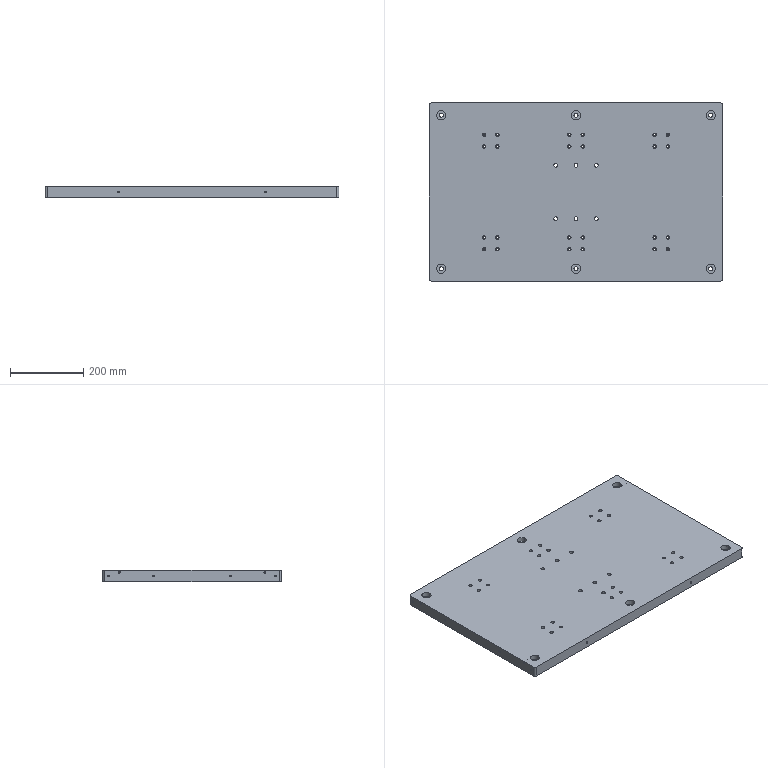NC program | Mastercam | posted with a generic post | part box 800 x 485 x 30 mm
Lines 4969 to 5776 of 13355:
N160 T9 M6
N170 G0 G90 G17 G54 X-108.24 Y-180.7 A0. S7000 M3
N180 G43 H9 Z50. M8
N190 Z1.
N200 G1 Z-.97 F600.
N210 Y-179.75 F3000.
N220 Y-173.741
N230 X-247.218
N240 Y-179.75
N250 G2 X-248.249 Y-180.781 I-1.031 J0.
N260 G1 X-252.509
N270 G2 X-253.541 Y-179.75 I0. J1.031
N280 G1 Y-167.418
N290 X-101.918
N300 Y-179.75
N310 G3 X-100.887 Y-180.781 I1.031 J0.
N320 G1 X-96.627
N330 G3 X-95.595 Y-179.75 I0. J1.031
N340 G1 Y-161.096
N350 X-259.863
N360 Y-179.75
N370 G2 X-260.894 Y-180.781 I-1.031 J0.
N380 G1 X-265.343
N390 G2 X-266.375 Y-179.75 I0. J1.031
N400 G1 X-266.374 Y-154.584
N410 X-89.084
N420 X-89.001 Y-179.75
N430 G3 X-87.972 Y-180.778 I1.031 J.003
N440 G1 X-83.604 Y-180.784
N450 X-83.602
N460 G3 X-82.571 Y-179.753 I0. J1.031
N470 G1 Y-179.75
N480 X-82.646 Y-152.389
N490 X-82.445 Y-148.147
N500 X-273.014
N510 X-272.812 Y-152.389
N520 X-272.888 Y-179.75
N530 G2 X-273.918 Y-180.778 I-1.031 J.003
N540 G1 X-278.098 Y-180.784
N550 X-278.099
N560 G2 X-279.131 Y-179.752 I0. J1.032
N570 G1 Y-179.75
N580 X-279.066 Y-152.389
N590 G3 X-280.436 Y-141.893 I-55.601 J-1.92
N600 G1 X-75.023
N610 G3 X-76.393 Y-152.389 I54.232 J-12.416
N620 G1 Y-179.75
N630 G3 X-75.361 Y-180.781 I1.032 J0.
N640 G1 X-71.477 Y-180.78
N650 G3 X-70.446 Y-179.75 I0. J1.032
N660 G1 X-70.396 Y-150.079
N670 G2 X-66.439 Y-135.985 I38.55 J-3.221
N680 G1 X-289.033
N690 G2 X-284.974 Y-152.389 I-33.033 J-16.878
N700 G1 X-285.029 Y-179.75
N710 G2 X-286.06 Y-180.779 I-1.031 J.002
N720 G1 X-289.089 Y-180.781
N730 G2 X-290.121 Y-179.75 I0. J1.031
N740 G1 X-290.12 Y-152.389
N750 G3 X-291.547 Y-143.256 I-54.5 J-3.836
N760 X-299.139 Y-130.838 I-30.518 J-10.127
N770 G1 X-56.319
N780 G3 X-65.338 Y-152.389 I21.751 J-21.766
N790 G1 X-65.262 Y-179.75
N800 Y-180.7
N810 G0 Z50.
N820 X98.24
N830 Z1.
N840 G1 Z-.97 F600.
N850 Y-179.75 F3000.
N860 Y-173.741
N870 X246.858
N880 Y-179.75
N890 G3 X247.889 Y-180.781 I1.031 J0.
N900 G1 X252.149
N910 G3 X253.18 Y-179.75 I0. J1.031
N920 G1 Y-167.418
N930 X91.918
N940 Y-179.75
N950 G2 X90.887 Y-180.781 I-1.031 J0.
N960 G1 X86.627
N970 G2 X85.595 Y-179.75 I0. J1.031
N980 G1 Y-161.096
N990 X259.503
N1000 Y-179.75
N1010 G3 X260.533 Y-180.781 I1.031 J0.
N1020 G1 X265.065 Y-180.785
N1030 X265.066
N1040 G3 X266.098 Y-179.753 I0. J1.032
N1050 G1 Y-179.75
N1060 X266.014 Y-154.584
N1070 X79.084
N1080 Y-179.75
N1090 G2 X78.053 Y-180.781 I-1.031 J0.
N1100 G1 X73.541 Y-180.782
N1110 G2 X72.51 Y-179.75 I0. J1.032
N1120 G1 X72.523 Y-149.152
N1130 X72.445 Y-148.147
N1140 X272.653
N1150 X272.452 Y-152.389
N1160 X272.527 Y-179.75
N1170 G3 X273.558 Y-180.778 I1.032 J.003
N1180 G1 X277.674 Y-180.781
N1190 G3 X278.705 Y-179.75 I0. J1.031
N1200 G1 Y-152.389
N1210 G2 X280.075 Y-141.893 I55.602 J-1.92
N1220 G1 X65.023
N1230 G2 X66.393 Y-152.389 I-54.232 J-12.416
N1240 G1 Y-179.75
N1250 G2 X65.362 Y-180.781 I-1.032 J0.
N1260 G1 X61.461 Y-180.783
N1270 G2 X60.43 Y-179.752 I0. J1.031
N1280 G1 Y-179.75
N1290 X60.484 Y-152.389
N1300 G3 X56.437 Y-135.985 I-37.292 J-.499
N1310 G1 X288.658
N1320 G3 X284.702 Y-150.079 I34.621 J-17.319
N1330 G1 X284.652 Y-179.75
N1340 Y-179.752
N1350 G3 X285.683 Y-180.783 I1.031 J0.
N1360 G1 X285.685
N1370 X288.785 Y-180.779
N1380 G3 X289.815 Y-179.75 I-.001 J1.031
N1390 G1 X289.887 Y-149.766
N1400 G2 X298.78 Y-130.838 I30.644 J-2.843
N1410 G1 X46.319
N1420 G2 X55.338 Y-152.389 I-21.719 J-21.752
N1430 G1 X55.262 Y-179.75
N1440 G2 X54.232 Y-180.778 I-1.031 J.003
N1450 G1 X51.99 Y-180.781
N1460 X51.989
N1470 G2 X50.958 Y-179.75 I0. J1.031
N1480 G1 Y-152.389
N1490 G3 X49.414 Y-143.661 I-37.021 J-2.047
N1500 X24.964 Y-126.458 I-24.45 J-8.773
N1510 G1 X24.706 Y-126.459
N1520 X-4.941 Y-126.458
N1530 X-35.55 Y-126.469
N1540 G3 X-45.618 Y-128.753 I1.584 J-30.309
N1550 X-60.958 Y-152.389 I10.663 J-23.716
N1560 G1 Y-179.75
N1570 G3 X-59.926 Y-180.781 I1.032 J0.
N1580 G1 X-56.231
N1590 G3 X-55.199 Y-179.75 I0. J1.031
N1600 G1 X-55.2 Y-152.389
N1610 G2 X-42.636 Y-133.739 I20.258 J-.089
N1620 X-35.479 Y-132.227 I8.822 J-24.062
N1630 G1 X-4.941 Y-132.217
N1640 X24.706
N1650 G2 X24.961 Y-132.215 I.255 J-20.226
N1660 X44.628 Y-147.712 I0. J-20.228
N1670 X45.2 Y-152.389 I-23.861 J-5.287
N1680 G1 X45.199 Y-179.75
N1690 G2 X44.168 Y-180.781 I-1.031 J0.
N1700 G1 X38.731
N1710 G2 X37.7 Y-179.75 I0. J1.031
N1720 G1 Y-152.389
N1730 X37.466 Y-150.05
N1740 G3 X24.945 Y-139.714 I-12.521 J-2.416
N1750 X24.706 Y-139.717 I0. J-12.752
N1760 G1 X-4.941
N1770 X-35.387 Y-139.726
N1780 G3 X-38.398 Y-140.192 I.7 J-14.491
N1790 X-47.7 Y-152.389 I3.468 J-12.29
N1800 G1 Y-179.75
N1810 G3 X-46.668 Y-180.781 I1.032 J0.
N1820 G1 X-41.231
N1830 G3 X-40.2 Y-179.75 I0. J1.031
N1840 G1 Y-152.389
N1850 G2 X-38.824 Y-148.893 I5.379 J-.098
N1860 X-36. Y-147.317 I3.89 J-3.654
N1870 G1 X-35.294 Y-147.225
N1880 X-34.589 Y-147.216
N1890 X-4.941
N1900 X24.706
N1910 G2 X24.915 Y-147.212 I.209 J-5.42
N1920 X28.236 Y-148.347 I0. J-5.424
N1930 X30.146 Y-151.683 I-3.335 J-4.125
N1940 G1 X30.2 Y-152.389
N1950 Y-179.8
N1960 G3 X30.208 Y-179.929 I1.031 J0.
N1970 X30.232 Y-180.056 I1.023 J.129
N1980 X30.272 Y-180.179 I.999 J.256
N1990 X30.327 Y-180.296 I.959 J.379
N2000 X30.396 Y-180.405 I.904 J.496
N2010 X30.478 Y-180.505 I.835 J.605
N2020 X30.572 Y-180.594 I.753 J.705
N2030 X30.677 Y-180.67 I.659 J.794
N2040 X30.79 Y-180.732 I.554 J.87
N2050 X30.91 Y-180.78 I.441 J.932
N2060 X31.035 Y-180.812 I.321 J.98
N2070 X31.163 Y-180.829 I.196 J1.012
N2080 X31.231 Y-180.831 I.068 J1.029
N2090 X31.293 Y-180.829 I0. J1.031
N2100 X31.421 Y-180.814 I-.062 J1.029
N2110 X31.546 Y-180.782 I-.19 J1.014
N2120 X31.667 Y-180.735 I-.315 J.982
N2130 G1 X31.741 Y-180.7
N2140 G0 Z50.
N2150 X110.882 Y180.7
N2160 Z1.
N2170 G1 Z-.97 F600.
N2180 Y179.75 F3000.
N2190 G2 X110.885 Y176.337 I-1974.811 J-3.873
N2200 G1 X130. Y173.396
N2210 X171.3 Y179.75
N2220 G3 X171.469 Y179.791 I-.156 J1.019
N2230 X171.628 Y179.859 I-.325 J.978
N2240 X171.773 Y179.953 I-.484 J.91
N2250 X171.901 Y180.07 I-.629 J.816
N2260 X172.008 Y180.206 I-.757 J.699
N2270 X172.09 Y180.359 I-.864 J.563
N2280 X172.145 Y180.523 I-.946 J.41
N2290 X172.172 Y180.694 I-1.001 J.246
N2300 G0 Z50.
N2310 X217.781
N2320 Z1.
N2330 G1 Z-.97 F600.
N2340 G3 X217.808 Y180.523 I1.028 J.075 F3000.
N2350 X217.863 Y180.359 I1.001 J.246
N2360 X217.945 Y180.206 I.946 J.41
N2370 X218.052 Y180.069 I.864 J.563
N2380 X218.179 Y179.953 I.757 J.7
N2390 X218.325 Y179.859 I.63 J.816
N2400 X218.484 Y179.791 I.484 J.91
N2410 X218.653 Y179.75 I.325 J.978
N2420 G1 X234.213 Y177.363
N2430 Y179.75
N2440 G2 X235.244 Y180.781 I1.031 J0.
N2450 G1 X239.504
N2460 G2 X240.535 Y179.75 I0. J-1.031
N2470 G1 Y169.994
N2480 X205.957 Y175.301
N2490 X197.254 Y176.019
N2500 G3 X182.812 Y175.124 I2.943 J-164.466
N2510 G1 X130. Y166.999
N2520 X104.563 Y170.913
N2530 Y179.75
N2540 G3 X103.532 Y180.781 I-1.031 J0.
N2550 G1 X99.272
N2560 G3 X98.24 Y179.75 I0. J-1.031
N2570 G1 Y165.488
N2580 X130. Y160.602
N2590 X183.774 Y168.875
N2600 G2 X197.048 Y169.7 I18.149 J-184.875
N2610 G1 X205.635 Y168.961
N2620 X246.858 Y162.624
N2630 Y179.75
N2640 G2 X247.889 Y180.781 I1.031 J0.
N2650 G1 X252.149
N2660 G2 X253.18 Y179.75 I0. J-1.031
N2670 G1 Y155.255
N2680 X204.749 Y162.701
N2690 X196.841 Y163.381
N2700 G3 X184.735 Y162.626 I8.881 J-239.961
N2710 G1 X130. Y154.205
N2720 X91.918 Y160.064
N2730 Y179.75
N2740 G3 X90.887 Y180.781 I-1.031 J0.
N2750 G1 X86.535 Y180.785
N2760 X86.534
N2770 G3 X85.503 Y179.754 I0. J-1.031
N2780 G1 Y179.75
N2790 X85.595 Y154.64
N2800 X130. Y147.808
N2810 X185.696 Y156.377
N2820 G2 X195.946 Y157.051 I10.25 J-77.614
N2830 X197.341 Y157.038 I0. J-78.288
N2840 G1 X203.862 Y156.441
N2850 X259.688 Y147.857
N2860 X259.58 Y179.75
N2870 Y180.7
N2880 G0 Z50.
N2890 X400.705 Y122.986
N2900 Z1.
N2910 G1 Z-.97 F600.
N2920 G3 X400.464 Y123.049 I-.383 J-.958 F3000.
N2930 X400.322 Y123.059 I-.142 J-1.021
N2940 X400.215 Y123.054 I0. J-1.031
N2950 X399.972 Y122.998 I.107 J-1.026
N2960 X399.75 Y122.886 I.35 J-.97
N2970 G2 X397.083 Y121.27 I-19.748 J29.59
N2980 X399.75 Y120.565 I-10.375 J-44.643
N2990 X400.47 Y119.766 I-.294 J-.989
N3000 G1 X401.109 Y116.344
N3010 G2 X401.127 Y116.154 I-1.013 J-.19
N3020 X400.096 Y115.123 I-1.031 J0.
N3030 X399.75 Y115.183 I0. J1.031
N3040 G3 X398.045 Y115.739 I-11.247 J-31.588
N3050 G1 X394.179 Y116.552
N3060 X358.259 Y122.078
N3070 G3 X364.193 Y122.05 I5.934 J638.917
N3080 X384.148 Y122.362 I0. J638.945
N3090 X395.65 Y126.383 I-5.237 J33.449
N3100 X399.75 Y129.33 I-15.663 J26.112
N3110 G2 X399.851 Y129.406 I.669 J-.785
N3120 X399.962 Y129.47 I.568 J-.861
N3130 X400.079 Y129.519 I.457 J-.925
N3140 X400.202 Y129.553 I.34 J-.974
N3150 X400.327 Y129.572 I.217 J-1.008
N3160 X400.419 Y129.576 I.092 J-1.027
N3170 G1 X400.455 Y129.575
N3180 G2 X400.581 Y129.564 I-.036 J-1.031
N3190 X400.705 Y129.536 I-.162 J-1.019
N3200 G0 Z50.
N3210 X400.7 Y-129.214
N3220 Z1.
N3230 G1 Z-.97 F600.
N3240 X400.181 Y-129.164 F3000.
N3250 G3 X400.082 Y-129.159 I-.099 J-1.026
N3260 X399.963 Y-129.166 I0. J-1.031
N3270 X399.75 Y-129.214 I.119 J-1.024
N3280 G2 X399.667 Y-129.242 I-9.786 J28.75
N3290 X399.75 Y-129.312 I-19.836 J-23.307
N3300 G3 X400.421 Y-129.56 I.671 J.783
N3310 X401.452 Y-128.529 I0. J1.031
N3320 X401.446 Y-128.419 I-1.031 J0.
N3330 G1 X401.12 Y-125.386
N3340 G3 X400.095 Y-124.465 I-1.025 J-.11
N3350 X399.75 Y-124.524 I0. J-1.031
N3360 G2 X390.731 Y-126.442 I-11.76 J33.139
N3370 G1 X350.121 Y-126.458
N3380 X-389.651
N3390 X-390.731 Y-126.442
N3400 G2 X-399.75 Y-124.545 I.751 J25.961
N3410 G3 X-399.882 Y-124.502 I-.388 J-.956
N3420 X-400.02 Y-124.476 I-.256 J-.999
N3430 X-400.138 Y-124.469 I-.118 J-1.025
N3440 X-400.159 Y-124.47 I0. J-1.032
N3450 X-400.298 Y-124.482 I.021 J-1.031
N3460 G1 X-400.7 Y-124.545
N3470 G0 Z50.
N3480 X-400.703 Y-135.412
N3490 Z1.
N3500 G1 Z-.97 F600.
N3510 G3 X-400.572 Y-135.427 I.186 J1.015 F3000.
N3520 X-400.517 Y-135.428 I.055 J1.03
N3530 X-400.441 Y-135.426 I0. J1.031
N3540 X-400.311 Y-135.408 I-.076 J1.029
N3550 X-400.184 Y-135.373 I-.206 J1.011
N3560 X-400.063 Y-135.323 I-.333 J.976
N3570 X-399.948 Y-135.258 I-.454 J.926
N3580 X-399.844 Y-135.179 I-.569 J.861
N3590 X-399.75 Y-135.087 I-.673 J.782
N3600 G2 X-392.359 Y-129.372 I19.351 J-17.391
N3610 X-382.009 Y-126.515 I12.84 J-26.338
N3620 G1 X-350.474 Y-126.458
N3630 X-320.474
N3640 G2 X-295.778 Y-144.408 I-.033 J-26.009
N3650 X-294.501 Y-152.389 I-33.54 J-9.461
N3660 G1 Y-179.75
N3670 G2 X-295.532 Y-180.781 I-1.031 J0.
N3680 G1 X-299.228
N3690 G2 X-300.259 Y-179.75 I0. J1.031
N3700 G1 Y-152.389
N3710 G3 X-301.195 Y-146.37 I-26.171 J-.99
N3720 X-320.474 Y-132.217 I-19.317 J-6.106
N3730 G1 X-350.474
N3740 X-381.583 Y-132.258
N3750 G3 X-387.964 Y-133.684 I2.393 J-25.69
N3760 X-399.75 Y-146.475 I7.557 J-18.789
N3770 G2 X-399.808 Y-146.623 I-.985 J.305
N3780 X-399.889 Y-146.76 I-.927 J.453
N3790 X-399.99 Y-146.884 I-.846 J.59
N3800 X-400.109 Y-146.99 I-.745 J.714
N3810 X-400.242 Y-147.076 I-.626 J.82
N3820 X-400.388 Y-147.141 I-.493 J.906
N3830 X-400.541 Y-147.183 I-.347 J.971
N3840 X-400.7 Y-147.201 I-.194 J1.013
N3850 G0 Z50.
N3860 X-393.483 Y-179.966
N3870 Z1.
N3880 G1 Z-.97 F600.
N3890 G3 X-393.346 Y-179.808 I-.706 J.751 F3000.
N3900 X-393.243 Y-179.624 I-.843 J.593
N3910 X-393.179 Y-179.424 I-.946 J.409
N3920 X-393.158 Y-179.215 I-1.01 J.209
N3930 G1 Y-152.389
N3940 G2 X-384.09 Y-140.256 I12.781 J-.098
N3950 X-380.474 Y-139.717 I4.113 J-15.189
N3960 G1 X-350.474
N3970 X-320.474
N3980 G2 X-307.993 Y-150.05 I-.036 J-12.747
N3990 G1 X-307.759 Y-152.389
N4000 Y-179.75
N4010 G2 X-308.781 Y-180.781 I-1.031 J0.
N4020 G1 X-314.218 Y-180.831
N4030 X-314.227
N4040 G2 X-315.259 Y-179.8 I0. J1.031
N4050 G1 Y-152.389
N4060 X-315.312 Y-151.683
N4070 G3 X-320.474 Y-147.216 I-5.163 J-.75
N4080 G1 X-350.474
N4090 X-380.474
N4100 X-381.18 Y-147.269
N4110 G3 X-385.658 Y-152.389 I.737 J-5.163
N4120 G1 Y-179.75
N4130 G2 X-385.669 Y-179.901 I-1.031 J0.
N4140 X-385.702 Y-180.049 I-1.02 J.151
N4150 X-385.757 Y-180.19 I-.987 J.299
N4160 X-385.831 Y-180.322 I-.932 J.44
N4170 X-385.924 Y-180.441 I-.858 J.572
N4180 X-386.033 Y-180.546 I-.765 J.691
N4190 X-386.157 Y-180.633 I-.656 J.796
N4200 X-386.292 Y-180.701 I-.532 J.883
N4210 G1 X-388.266 Y-181.527
N4220 G0 Z50.
N4230 X-400.7 Y120.617
N4240 Z1.
N4250 G1 Z-.97 F600.
N4260 X-400.099 Y120.579 F3000.
N4270 G3 X-400.034 Y120.577 I.065 J1.029
N4280 X-399.923 Y120.583 I0. J1.031
N4290 X-399.75 Y120.617 I-.111 J1.025
N4300 G2 X-397.32 Y121.221 I9.78 J-34.13
N4310 G1 X-399.75 Y122.846
N4320 G2 X-400.172 Y123.434 I.573 J.857
N4330 G1 X-401.402 Y127.978
N4340 G2 X-401.438 Y128.247 I.995 J.269
N4350 X-400.407 Y129.278 I1.031 J0.
N4360 X-399.75 Y129.042 I0. J-1.031
N4370 G3 X-389.358 Y123.422 I19.445 J23.538
N4380 X-382.333 Y122.147 I10.313 J36.823
N4390 G1 X-358.258 Y122.078
N4400 X-395.15 Y116.394
N4410 G3 X-399.75 Y115.044 I32.279 J-118.497
N4420 G2 X-399.943 Y115.003 I-.309 J.983
N4430 X-400.059 Y114.996 I-.116 J1.024
N4440 X-400.141 Y114.999 I0. J1.031
N4450 G1 X-400.7 Y115.044
N4460 G0 Z50.
N4470 X-234.577 Y180.7
N4480 Z1.
N4490 G1 Z-.97 F600.
N4500 Y179.75 F3000.
N4510 G2 X-234.573 Y177.308 I-2046.876 J-4.537
N4520 G1 X-218.652 Y179.75
N4530 G3 X-218.484 Y179.791 I-.157 J1.019
N4540 X-218.325 Y179.859 I-.325 J.978
N4550 X-218.179 Y179.953 I-.484 J.91
N4560 X-218.051 Y180.069 I-.63 J.816
N4570 X-217.945 Y180.206 I-.758 J.7
N4580 X-217.863 Y180.359 I-.864 J.563
N4590 X-217.807 Y180.523 I-.946 J.41
N4600 X-217.78 Y180.694 I-1.002 J.246
N4610 G0 Z50.
N4620 X-172.933 Y180.693
N4630 Z1.
N4640 G1 Z-.97 F600.
N4650 G3 X-172.905 Y180.522 I1.029 J.077 F3000.
N4660 X-172.85 Y180.358 I1.001 J.248
N4670 X-172.767 Y180.205 I.946 J.412
N4680 X-172.661 Y180.069 I.863 J.565
N4690 X-172.532 Y179.952 I.757 J.701
N4700 X-172.386 Y179.858 I.628 J.818
N4710 X-172.227 Y179.79 I.482 J.912
N4720 X-172.058 Y179.75 I.323 J.98
N4730 G1 X-130. Y173.396
N4740 X-120.885 Y174.798
N4750 Y179.75
N4760 G2 X-119.854 Y180.781 I1.031 J0.
N4770 G1 X-115.594
N4780 G2 X-114.563 Y179.75 I0. J-1.031
N4790 G1 Y169.374
N4800 X-130. Y166.999
N4810 X-182.812 Y175.124
N4820 G3 X-197.255 Y176.019 I-17.381 J-163.519
N4830 G1 X-205.957 Y175.301
N4840 X-240.896 Y169.938
N4850 Y179.75
N4860 G3 X-241.927 Y180.781 I-1.031 J0.
N4870 G1 X-246.187
N4880 G3 X-247.218 Y179.75 I0. J-1.031
N4890 G1 Y162.569
N4900 X-205.635 Y168.961
N4910 X-197.048 Y169.7
N4920 G2 X-183.774 Y168.875 I-4.869 J-185.617
N4930 G1 X-130. Y160.602
N4940 X-108.24 Y163.95
N4950 Y179.75
N4960 G2 X-107.209 Y180.781 I1.031 J0.
N4970 G1 X-102.949
N4980 G2 X-101.918 Y179.75 I0. J-1.031
N4990 G1 Y158.526
N5000 X-130. Y154.205
N5010 X-184.735 Y162.626
N5020 G3 X-196.842 Y163.381 I-20.975 J-239.027
N5030 G1 X-204.749 Y162.701
N5040 X-253.54 Y155.199
N5050 X-253.541 Y179.75
N5060 G3 X-254.572 Y180.781 I-1.031 J0.
N5070 G1 X-259.023
N5080 G3 X-260.054 Y179.75 I0. J-1.031
N5090 G1 X-260.051 Y147.816
N5100 X-260.001 Y147.809
N5110 X-203.863 Y156.441
N5120 X-196.635 Y157.062
N5130 G2 X-196.112 Y157.064 I.523 J-79.4
N5140 X-185.696 Y156.377 I0. J-79.402
N5150 G1 X-130. Y147.808
N5160 X-95.595 Y153.101
N5170 Y179.75
N5180 G2 X-94.564 Y180.781 I1.031 J0.
N5190 G1 X-90.115
N5200 G2 X-89.084 Y179.75 I0. J-1.031
N5210 G1 Y152.389
N5220 X-88.855 Y147.55
N5230 X-130. Y141.22
N5240 X-186.686 Y149.941
N5250 G3 X-195.929 Y150.555 I-9.243 J-69.264
N5260 X-196.423 Y150.554 I0. J-69.878
N5270 G1 X-202.95 Y149.994
N5280 X-260.001 Y141.221
N5290 X-267.328 Y142.348
N5300 G3 X-266.374 Y152.389 I-276.809 J31.355
N5310 G1 X-266.375 Y179.75
N5320 G3 X-267.406 Y180.781 I-1.031 J0.
N5330 G1 X-271.781
N5340 G3 X-272.812 Y179.75 I0. J-1.031
N5350 G1 Y152.389
N5360 G2 X-275.362 Y137.07 I-54.972 J1.28
N5370 G1 X-260.001 Y134.707
N5380 X-202.047 Y143.62
N5390 X-196.212 Y144.119
N5400 X-187.665 Y143.579
N5410 X-130. Y134.707
N5420 X-81.513 Y142.167
N5430 G2 X-82.646 Y152.389 I119.977 J18.478
N5440 G1 X-82.542 Y179.75
N5450 Y180.7
N5460 G0 Z50.
N5470 X78.94
N5480 Z1.
N5490 G1 Z-.97 F600.
N5500 Y179.75 F3000.
N5510 X78.971 Y149.071
N5520 X130. Y141.22
N5530 X186.686 Y149.941
N5540 G2 X195.799 Y150.543 I9.113 J-68.676
N5550 X197.128 Y150.531 I0. J-69.278
N5560 G1 X203.529 Y149.908
N5570 X260.001 Y141.221
N5580 X266.978 Y142.294
N5590 G2 X266.014 Y152.389 I255.574 J29.502
N5600 G1 Y179.75
N5610 G2 X267.046 Y180.781 I1.032 J0.
N5620 G1 X271.474 Y180.779
N5630 G2 X272.505 Y179.75 I-.001 J-1.031
N5640 G1 X272.575 Y149.152
N5650 G3 X275.024 Y137.018 I63.263 J6.454
N5660 G1 X260.001 Y134.707
N5670 X202.55 Y143.546
N5680 X196.918 Y144.096
N5690 G3 X195.659 Y144.109 I-1.259 J-60.445
N5700 X187.665 Y143.579 I0. J-60.458
N5710 G1 X130. Y134.707
N5720 X71.826 Y143.654
N5730 X72.646 Y152.389
N5740 Y179.75
N5750 G3 X71.615 Y180.781 I-1.031 J0.
N5760 G1 X67.424
N5770 G3 X66.393 Y179.75 I0. J-1.031
N5780 G1 Y152.389
N5790 G2 X63.727 Y137.87 I-45.867 J.919
N5800 G1 X70.986 Y137.456
N5810 X130. Y128.38
N5820 X188.616 Y137.398
N5830 G2 X195.53 Y137.86 I6.914 J-51.528
N5840 X196.713 Y137.846 I0. J-51.99
N5850 G1 X201.599 Y137.365
N5860 X260.001 Y128.38
N5870 X284.056 Y132.081
N5880 G2 X278.811 Y149.629 I38.334 J21.016
N5890 G1 X278.853 Y179.75
N5900 G2 X279.884 Y180.78 I1.032 J-.001
N5910 G1 X283.711 Y180.783
N5920 X283.712
N5930 G2 X284.744 Y179.751 I0. J-1.032
N5940 G1 Y179.75
N5950 X284.702 Y150.079
N5960 G3 X289.601 Y134.297 I37.521 J2.995
N5970 X294.613 Y127.727 I37.93 J23.739
N5980 G1 X260.001 Y122.402
N5990 X200.701 Y131.525
N6000 G3 X195.815 Y131.964 I-6.07 J-40.141
N6010 G1 X189.515 Y131.558
N6020 X130. Y122.402
N6030 X70.115 Y131.613
N6040 G3 X64.921 Y131.857 I-5.194 J-55.23
N6050 X52.934 Y130.546 I0. J-55.474
N6060 X60.342 Y149.374 I-28.869 J22.23
N6070 G1 X60.362 Y179.75
N6080 Y179.751
N6090 G3 X59.332 Y180.782 I-1.031 J0.
N6100 G1 X56.294 Y180.784
N6110 X56.293
N6120 G3 X55.262 Y179.753 I0. J-1.031
N6130 G1 Y179.75
N6140 X55.338 Y152.389
N6150 G2 X53.513 Y142.117 I-38.612 J1.561
N6160 X29.234 Y122.388 I-28.523 J10.297
N6170 G1 X24.706 Y122.078
N6180 X-31.742
N6190 X0. Y117.195
N6200 X60.413 Y126.489
N6210 X66.299 Y126.799
N6220 X130. Y117.195
N6230 X190.297 Y126.471
N6240 X195.646 Y126.82
N6250 G2 X199.918 Y126.438 I-.95 J-34.712
N6260 G1 X260.001 Y117.195
N6270 X308.072 Y124.591
N6280 G2 X290.575 Y145.504 I12.019 J27.831
N6290 X289.76 Y152.389 I37.162 J7.887
N6300 G1 Y179.75
N6310 G2 X290.792 Y180.781 I1.032 J0.
N6320 G1 X291.368
N6330 G2 X292.399 Y179.75 I0. J-1.031
N6340 G1 Y152.389
N6350 G3 X294.054 Y143.047 I37.433 J1.816
N6360 X320.136 Y124.715 I26.082 J9.388
N6370 X320.474 Y124.717 I0. J27.72
N6380 G1 X324.709
N6390 X380.925 Y124.736
N6400 G3 X389.036 Y126.212 I-2.361 J35.991
N6410 X399.75 Y132.922 I-8.983 J26.25
N6420 G2 X399.847 Y133.008 I.732 J-.726
N6430 X399.954 Y133.081 I.635 J-.812
N6440 X400.069 Y133.141 I.528 J-.885
N6450 X400.191 Y133.185 I.413 J-.945
N6460 X400.317 Y133.214 I.291 J-.989
N6470 X400.446 Y133.226 I.165 J-1.018
N6480 X400.482 Y133.227 I.036 J-1.03
N6490 X400.576 Y133.223 I0. J-1.031
N6500 X400.704 Y133.203 I-.094 J-1.027
N6510 G0 Z50.
N6520 X400.699 Y148.572
N6530 Z1.
N6540 G1 Z-.97 F600.
N6550 G3 X400.535 Y148.55 I.054 J-1.029 F3000.
N6560 X400.376 Y148.502 I.218 J-1.007
N6570 X400.228 Y148.43 I.377 J-.959
N6580 X400.092 Y148.334 I.525 J-.887
N6590 X399.974 Y148.219 I.661 J-.791
N6600 X399.876 Y148.085 I.779 J-.676
N6610 X399.801 Y147.938 I.877 J-.542
N6620 X399.75 Y147.781 I.952 J-.395
N6630 G2 X385.074 Y132.849 I-19.694 J4.679
N6640 G1 X380.069 Y132.22
N6650 X324.709 Y132.217
N6660 X320.474
N6670 G2 X320.144 Y132.214 I-.33 J20.234
N6680 X300.47 Y147.712 I0. J20.237
N6690 X299.899 Y152.389 I23.861 J5.287
N6700 G1 Y179.75
N6710 G2 X300.93 Y180.781 I1.031 J0.
N6720 G1 X306.367
N6730 G2 X307.399 Y179.75 I0. J-1.031
N6740 G1 X307.398 Y152.389
N6750 X307.632 Y150.05
N6760 G3 X320.16 Y139.712 I12.528 J2.422
N6770 X320.474 Y139.717 I0. J12.76
N6780 G1 X324.709
N6790 X382.276 Y139.916
N6800 G3 X392.798 Y152.389 I-2.22 J12.547
N6810 G1 Y179.323
N6820 G3 X391.852 Y180.351 I-1.031 J0.
N6830 G1 X386.415 Y180.802
N6840 G3 X386.329 Y180.806 I-.086 J-1.027
N6850 X385.298 Y179.775 I0. J-1.031
N6860 G1 Y152.389
N6870 G2 X383.893 Y148.861 I-5.376 J.098
N6880 X380.474 Y147.231 I-3.867 J3.708
N6890 G1 X324.709 Y147.216
N6900 X320.474
N6910 G2 X320.196 Y147.209 I-.278 J5.449
N6920 X316.944 Y148.284 I0. J5.456
N6930 X314.952 Y151.683 I3.241 J4.183
N6940 G1 X314.898 Y152.389
N6950 Y179.75
N6960 G3 X314.871 Y179.988 I-1.031 J0.
N6970 X314.789 Y180.212 I-1.004 J-.238
N6980 X314.658 Y180.412 I-.922 J-.462
N6990 X314.484 Y180.577 I-.791 J-.662
N7000 X314.277 Y180.696 I-.617 J-.827
N7010 X314.048 Y180.765 I-.41 J-.946
N7020 X313.867 Y180.781 I-.181 J-1.015
N7030 X313.809 Y180.78 I0. J-1.031
N7040 X313.573 Y180.738 I.058 J-1.03
N7050 G1 X313.444 Y180.7
N7060 G0 Z50.
N7070 X400.702 Y-118.05
N7080 Z1.
N7090 G1 Z-.97 F600.
N7100 G3 X400.468 Y-117.969 I-.452 J-.927 F3000.
N7110 X400.25 Y-117.946 I-.218 J-1.008
N7120 G1 X400.223
N7130 G3 X399.978 Y-117.982 I.027 J-1.031
N7140 X399.75 Y-118.075 I.272 J-.995
N7150 G2 X396.004 Y-119.684 I-9.791 J17.627
N7160 X390.626 Y-120.606 I-6.865 J23.905
N7170 G1 X350.121 Y-120.621
N7180 X-389.651
N7190 X-390.626 Y-120.606
N7200 G2 X-399.75 Y-118.086 I.651 J20.131
N7210 G3 X-399.978 Y-117.992 I-.5 J-.901
N7220 X-400.223 Y-117.956 I-.272 J-.995
N7230 G1 X-400.25
N7240 G3 X-400.468 Y-117.979 I0. J-1.031
N7250 X-400.702 Y-118.06 I.218 J-1.008
N7260 G0 Z50.
N7270 X-279.182 Y180.7
N7280 Z1.
N7290 G1 Z-.97 F600.
N7300 Y179.75 F3000.
N7310 X-279.171 Y149.629
N7320 G2 X-284.396 Y132.133 I-42.705 J3.227
N7330 G1 X-260.001 Y128.38
N7340 X-201.599 Y137.365
N7350 X-196.008 Y137.869
N7360 X-188.616 Y137.398
N7370 X-130. Y128.38
N7380 X-73.427 Y137.083
N7390 G2 X-76.393 Y152.389 I42.062 J16.091
N7400 G1 Y179.75
N7410 G2 X-75.361 Y180.781 I1.032 J0.
N7420 G1 X-71.454 Y180.778
N7430 G2 X-70.423 Y179.75 I-.001 J-1.031
N7440 G1 X-70.342 Y149.374
N7450 G3 X-63.99 Y131.967 I36.632 J3.506
N7460 G1 X-70.115 Y131.613
N7470 X-130. Y122.402
N7480 X-189.515 Y131.558
N7490 X-195.815 Y131.964
N7500 X-200.701 Y131.525
N7510 X-260.001 Y122.402
N7520 X-294.926 Y127.775
N7530 G3 X-285.116 Y149.374 I-26.09 J24.877
N7540 G1 X-285.035 Y179.75
N7550 Y179.753
N7560 G3 X-286.066 Y180.784 I-1.031 J0.
N7570 G1 X-286.067
N7580 X-289.09 Y180.781
N7590 G3 X-290.121 Y179.75 I.001 J-1.031
N7600 G1 X-290.12 Y152.389
N7610 X-290.778 Y146.21
N7620 G2 X-308.318 Y124.629 I-29.741 J6.254
N7630 G1 X-260.001 Y117.195
N7640 X-199.918 Y126.438
N7650 X-196.353 Y126.797
N7660 G2 X-195.322 Y126.811 I1.031 J-37.298
N7670 X-190.297 Y126.471 I0. J-37.312
N7680 G1 X-130. Y117.195
N7690 X-69.919 Y126.438
N7700 X-67.005 Y126.761
N7710 G2 X-65.273 Y126.8 I1.732 J-38.089
N7720 X-60.414 Y126.489 I0. J-38.128
N7730 G1 X-46.44 Y124.34
N7740 G2 X-64.681 Y146.21 I11.454 J28.095
N7750 G1 X-65.338 Y152.389
N7760 Y179.75
N7770 G2 X-64.307 Y180.781 I1.031 J0.
N7780 G1 X-63.73
N7790 G2 X-62.699 Y179.75 I0. J-1.031
N7800 G1 Y152.389
N7810 G3 X-61.044 Y143.047 I37.432 J1.816
N7820 X-39.422 Y125.08 I26.094 J9.407
N7830 X-34.589 Y124.717 I4.962 J33.724
N7840 G1 X24.706
N7850 G3 X32.039 Y125.637 I-.89 J36.793
N7860 X52.58 Y149.968 I-7.055 J26.792
N7870 G1 X52.647 Y179.75
N7880 Y179.752
N7890 G3 X51.616 Y180.783 I-1.031 J0.
N7900 G1 X51.615
N7910 X46.187 Y180.779
N7920 G3 X45.157 Y179.75 I.001 J-1.031
N7930 G1 X45.102 Y150.54
N7940 G2 X30.065 Y132.872 I-20.132 J1.901
N7950 X24.706 Y132.217 I-5.794 J25.142
N7960 G1 X-34.589
N7970 X-34.593
N7980 G2 X-38.281 Y132.492 I0. J24.819
N7990 X-54.628 Y147.712 I3.328 J19.964
N8000 X-55.2 Y152.389 I23.861 J5.287
N8010 G1 X-55.199 Y179.75
N8020 G2 X-54.168 Y180.781 I1.031 J0.
N8030 G1 X-48.731
N8040 G2 X-47.7 Y179.75 I0. J-1.031
N8050 G1 Y152.389
N8060 X-47.466 Y150.05
N8070 G3 X-37.141 Y139.905 I12.533 J2.428
N8080 G1 X-35.387 Y139.726
N8090 X26.552 Y139.821
N8100 G3 X37.624 Y151.111 I-1.592 J12.635
N8110 G1 X37.666 Y179.75
N8120 Y179.752
N8130 G3 X36.644 Y180.783 I-1.031 J0.
N8140 G1 X31.24 Y180.831
N8150 X31.231
N8160 G3 X30.2 Y179.8 I0. J-1.031
N8170 G1 Y152.389
N8180 X30.146 Y151.683
N8190 G2 X28.795 Y148.861 I-5.397 J.85
N8200 X25.412 Y147.233 I-3.869 J3.712
N8210 G1 X-34.589 Y147.216
N8220 X-35.294 Y147.225
N8230 X-36. Y147.317